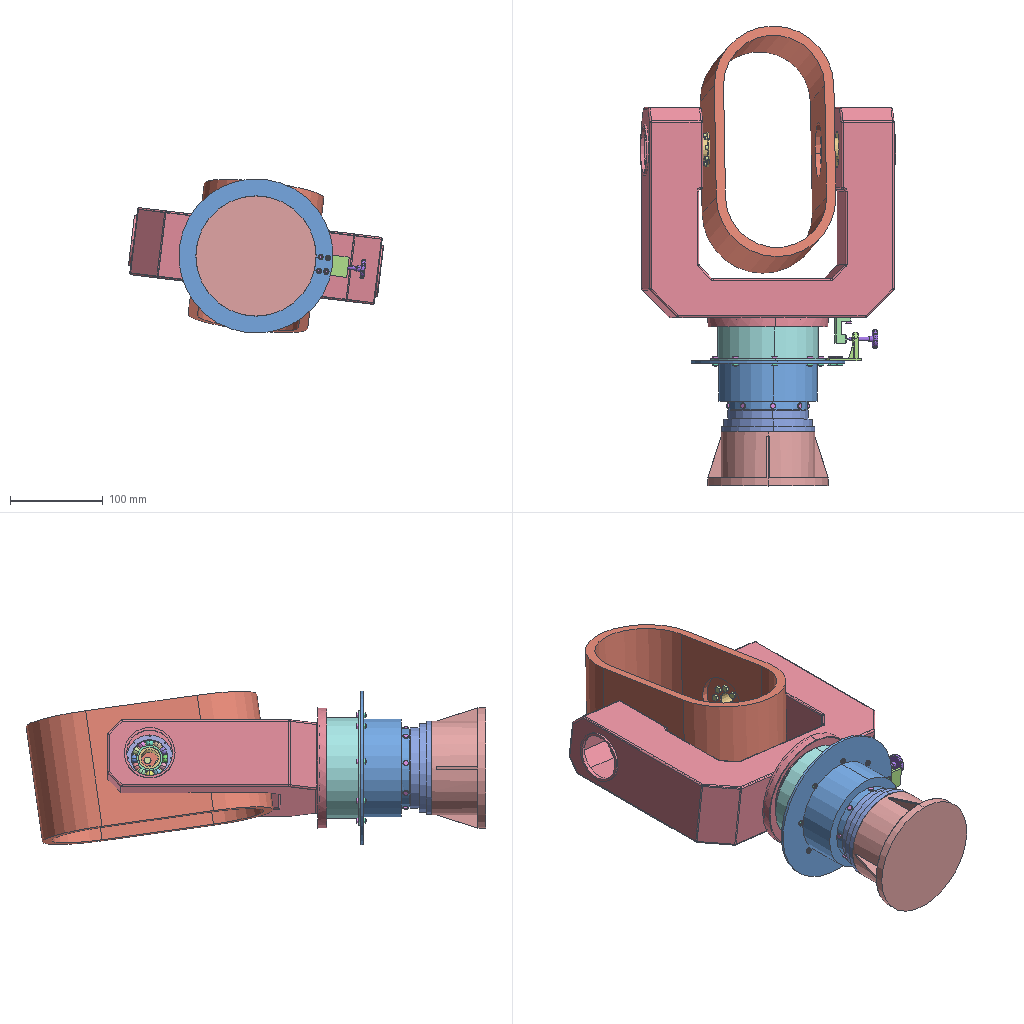Assembly | SolidWorks | 20 different items | 23 placed | box 276 x 497 x 166 mm
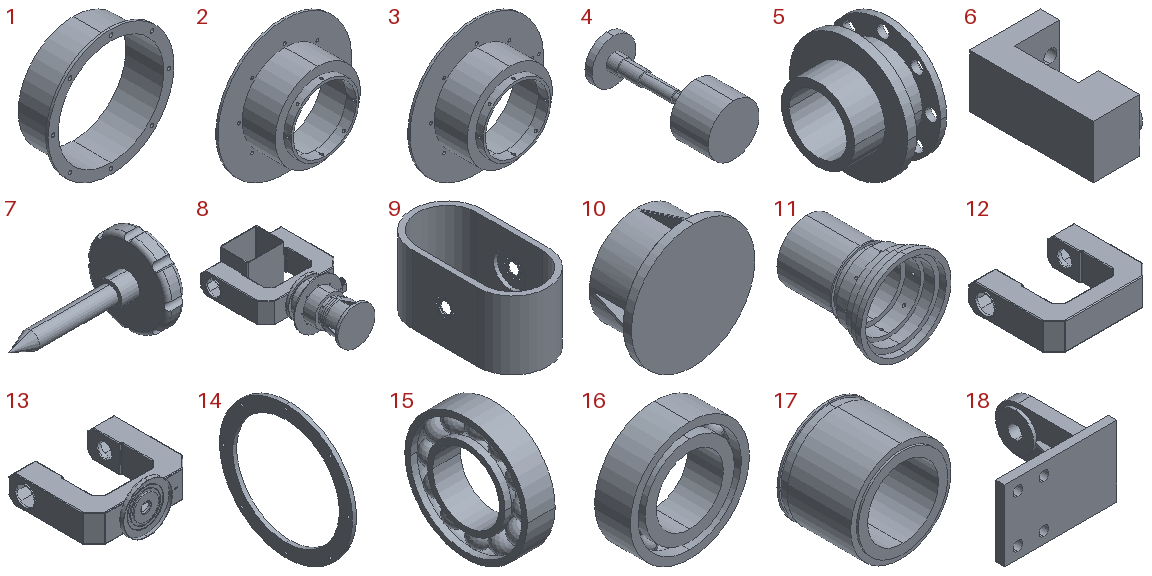Parts list (item | name | quantity | size | volume | features):
1 | - | x1 | 124.775 x 37.645 x 124.775 mm | 33353 mm3 | features SavedExtBody 1
2 | - | x1 | 166.652 x 52.651 x 166.652 mm | 97118 mm3 | features SavedExtBody 1
3 | - | x1 | 166.652 x 52.651 x 166.652 mm | 97043 mm3 | features SavedExtBody 1
4 | - | x1 | 67.426 x 169.265 x 67.426 mm | 221151 mm3 | features SavedExtBody 1
5 | - | x2 | 24.772 x 38.609 x 38.609 mm | 8203 mm3 | features SavedExtBody 1
6 | - | x1 | 15.948 x 27.791 x 12 mm | 2925 mm3 | features SavedExtBody 1
7 | - | x1 | 33.456 x 20.157 x 20.157 mm | 1733 mm3 | features SavedExtBody 1
8 | - | x1 | 271.015 x 413.124 x 166.652 mm | 1725111 mm3 | features ICE 33, Revolution 14, CirPattern 5, RevCut 3, Shell 2, Chamfer 1, Extrusion 1, Fillet 1, MirrorPattern 1, RefAxis 1
9 | - | x1 | 130 x 251.564 x 126.792 mm | 744560 mm3 | features ICE 4, SavedExtBody 1
10 | - | x1 | 129.827 x 58.73 x 129.827 mm | 343940 mm3 | features SavedExtBody 1
11 | - | x1 | 101.384 x 111.36 x 101.384 mm | 137958 mm3 | features SavedExtBody 1
12 | - | x1 | 271.015 x 226.948 x 73 mm | 430356 mm3 | features SavedExtBody 1
13 | - | x1 | 271.015 x 236.948 x 130 mm | 273992 mm3 | features MoveFace 1, SavedExtBody 1
14 | - | x2 | 1.5 x 50 x 50 mm | 1051 mm3 | features SavedExtBody 1
15 | - | x2 | 10 x 44 x 44 mm | 6715 mm3 | features SavedExtBody 14
16 | - | x1 | 31.502 x 9.43 x 31.502 mm | 3555 mm3 | features SavedExtBody 14
17 | - | x1 | 95 x 71.846 x 95 mm | 199181 mm3 | features SavedExtBody 38
18 | - | x1 | 34.775 x 30.759 x 22 mm | 3678 mm3 | features SavedExtBody 1
19 | hex nuts, style 1-grades ab gb | x1 | - | - | -
20 | hexagon head bolts-full thread gb | x1 | - | - | -
Mates (type | each side: item.copy, entity, surface, feature):
Concentric | 10.1 face cylinder Base part-Part1-1 | 4.1 face cylinder Base part-Part1-1
Coincident | 10.1 face plane Base part-Part1-1 | 4.1 face plane Base part-Part1-1
Concentric | 11.1 face cylinder Base part-Part1-1 | 16.1 face cylinder Base part-Part1-12
Concentric | 4.1 face cylinder Base part-Part1-1 | 13.1 face cylinder Base part-Part1-1
Coincident | 4.1 face plane Base part-Part1-1 | 13.1 face plane Base part-Part1-1
Coincident | 17.1 face plane Base part-Part1-37 | 13.1 face plane Base part-Part1-1
Concentric | 17.1 face cylinder Base part-Part1-37 | 13.1 face cylinder Base part-Part1-1
Coincident | 10.1 face plane Base part-Part1-1 | 11.1 face plane Base part-Part1-1
Coincident | 11.1 face plane Base part-Part1-1 | 16.1 face plane Base part-Part1-12
Concentric | 11.1 face cylinder Base part-Part1-1 | 17.1 face cylinder Base part-Part1-37
Concentric | 17.1 face cylinder Base part-Part1-37 | 1.1 face cylinder Base part-Part1-1
Coincident | 9.1 face plane Base part-Part1-1 | 5.1 face plane Base part-Part1-1
Concentric | 9.1 face cylinder Base part-Part1-1 | 5.1 face cylinder Base part-Part1-1 | 2 times
Coincident | 15.1 face plane Base part-Part1-13 | 13.1 face plane Base part-Part1-1
Concentric | 15.1 face cylinder Base part-Part1-13 | 13.1 face cylinder Base part-Part1-1
Coincident | 15.1 face plane Base part-Part1-14 | 5.1 face plane Base part-Part1-1
Concentric | 5.1 face cylinder Base part-Part1-1 | 13.1 face cylinder Base part-Part1-1
Coincident | 14.1 face plane Base part-Part1-1 | 13.1 face plane Base part-Part1-1
Concentric | 14.1 face cylinder Base part-Part1-1 | 13.1 face cylinder Base part-Part1-1
Coincident | 1.1 face plane Base part-Part1-1 | 3.1 face plane Base part-Part1-1
Concentric | 1.1 face cylinder Base part-Part1-1 | 3.1 face cylinder Base part-Part1-1 | 2 times
Coincident | 18.1 face plane Base part-Part1-1 | 3.1 face plane Base part-Part1-1
Concentric | 18.1 face cylinder Base part-Part1-1 | 3.1 face cylinder Base part-Part1-1 | 2 times
Coincident | 6.1 face plane Base part-Part1-1 | 13.1 face plane Base part-Part1-1
Concentric | 6.1 face cylinder Base part-Part1-1 | 13.1 face cylinder Base part-Part1-1 | 2 times
Coincident | 9.1 face plane Base part-Part1-1 | 5.2 face plane Base part-Part1-1
Concentric | 13.1 face cylinder Base part-Part1-1 | 5.2 face cylinder Base part-Part1-1
Concentric | 9.1 face cylinder Base part-Part1-1 | 5.2 face cylinder Base part-Part1-1
Coincident | 13.1 face plane Base part-Part1-1 | 15.2 face plane Base part-Part1-13
Concentric | 13.1 face cylinder Base part-Part1-1 | 15.2 face cylinder Base part-Part1-13
Coincident | 13.1 face plane Base part-Part1-1 | 14.2 face plane Base part-Part1-1
Concentric | 13.1 face cylinder Base part-Part1-1 | 14.2 face cylinder Base part-Part1-1
Concentric | 7.1 face cylinder Base part-Part1-1 | 6.1 face cylinder Base part-Part1-1
Concentric | 11.1 face cylinder Base part-Part1-1 | 3.1 face cylinder Base part-Part1-1
Concentric | 18.1 face cylinder Base part-Part1-1 | 7.1 edge
Concentric | 18.1 edge | 7.1 edge
Lock | 18.1 select_type:0 | 7.1 select_type:0